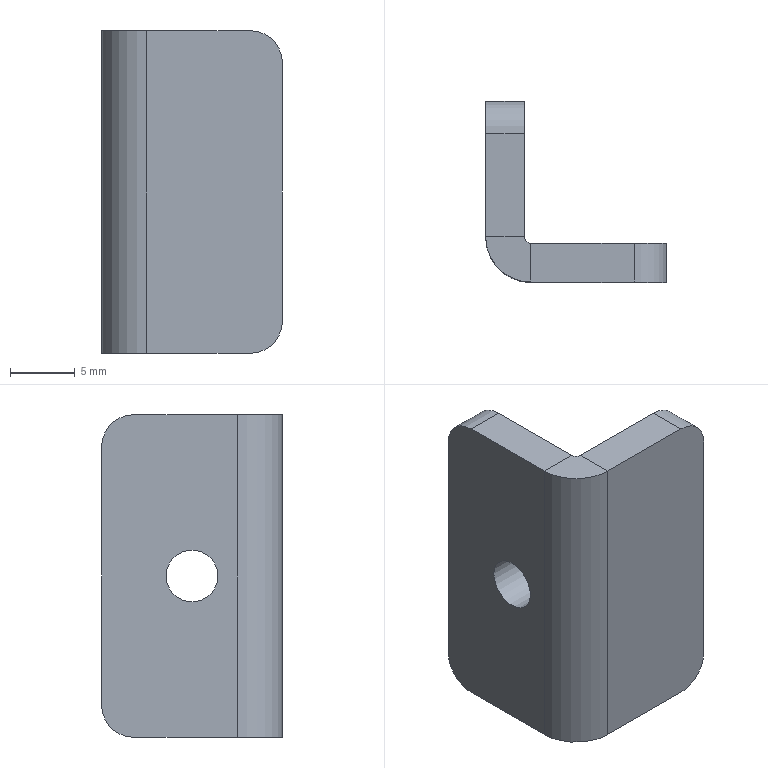Part | STEP file | Q7C0513 | 1 solid | 19 faces | box 14 x 14 x 25 mm | volume 1757 mm3 | plane 12 | cylinder 7 | commonest cylinder face diameters 5 x4 1 x1 4 x1 7 x1
STEP:
#1=CARTESIAN_POINT('',(0.,0.,0.));
#2=DIRECTION('',(0.,0.,1.));
#3=DIRECTION('',(1.,0.,0.));
#4=AXIS2_PLACEMENT_3D('',#1,#2,#3);
#5=CARTESIAN_POINT('',(0.,3.5,12.5));
#6=VERTEX_POINT('',#5);
#7=CARTESIAN_POINT('',(3.,3.5,12.5));
#8=VERTEX_POINT('',#7);
#9=CARTESIAN_POINT('',(0.,3.5,12.5));
#10=DIRECTION('',(1.,0.,0.));
#11=VECTOR('',#10,1.);
#12=LINE('',#9,#11);
#13=CARTESIAN_POINT('',(0.,3.5,12.5));
#14=DIRECTION('',(0.,0.,1.));
#15=DIRECTION('',(1.,0.,0.));
#16=AXIS2_PLACEMENT_3D('',#13,#14,#15);
#17=PLANE('',#16);
#18=CARTESIAN_POINT('',(0.,0.));
#19=DIRECTION('',(1.,0.));
#20=VECTOR('',#19,1.);
#21=LINE('',#18,#20);
#22=(GEOMETRIC_REPRESENTATION_CONTEXT(2)PARAMETRIC_REPRESENTATION_CONTEXT()REPRESENTATION_CONTEXT('',''));
#23=DEFINITIONAL_REPRESENTATION('',(#21),#22);
#24=PCURVE('',#17,#23);
#25=CARTESIAN_POINT('',(3.5,3.,12.5));
#26=DIRECTION('',(0.,0.,1.));
#27=DIRECTION('',(1.,0.,0.));
#28=AXIS2_PLACEMENT_3D('',#25,#26,#27);
#29=PLANE('',#28);
#30=CARTESIAN_POINT('',(-3.5,0.5));
#31=DIRECTION('',(1.,0.));
#32=VECTOR('',#31,1.);
#33=LINE('',#30,#32);
#34=(GEOMETRIC_REPRESENTATION_CONTEXT(2)PARAMETRIC_REPRESENTATION_CONTEXT()REPRESENTATION_CONTEXT('',''));
#35=DEFINITIONAL_REPRESENTATION('',(#33),#34);
#36=PCURVE('',#29,#35);
#37=SURFACE_CURVE('',#12,(#24,#36),.PCURVE_S1.);
#38=EDGE_CURVE('',#6,#8,#37,.T.);
#39=ORIENTED_EDGE('',*,*,#38,.F.);
#40=CARTESIAN_POINT('',(3.5,0.,12.5));
#41=VERTEX_POINT('',#40);
#42=CARTESIAN_POINT('',(3.5,3.5,12.5));
#43=DIRECTION('',(0.,0.,1.));
#44=DIRECTION('',(-1.,0.,0.));
#45=AXIS2_PLACEMENT_3D('',#42,#43,#44);
#46=CIRCLE('',#45,3.5);
#47=CARTESIAN_POINT('',(3.5,0.));
#48=DIRECTION('',(-1.,0.));
#49=AXIS2_PLACEMENT_2D('',#47,#48);
#50=CIRCLE('',#49,3.5);
#51=(GEOMETRIC_REPRESENTATION_CONTEXT(2)PARAMETRIC_REPRESENTATION_CONTEXT()REPRESENTATION_CONTEXT('',''));
#52=DEFINITIONAL_REPRESENTATION('',(#50),#51);
#53=PCURVE('',#17,#52);
#54=CARTESIAN_POINT('',(3.5,3.5,12.5));
#55=DIRECTION('',(0.,0.,-1.));
#56=DIRECTION('',(-1.,0.,0.));
#57=AXIS2_PLACEMENT_3D('',#54,#55,#56);
#58=CYLINDRICAL_SURFACE('',#57,3.5);
#59=CARTESIAN_POINT('',(6.283,0.));
#60=DIRECTION('',(-1.,0.));
#61=VECTOR('',#60,1.);
#62=LINE('',#59,#61);
#63=(GEOMETRIC_REPRESENTATION_CONTEXT(2)PARAMETRIC_REPRESENTATION_CONTEXT()REPRESENTATION_CONTEXT('',''));
#64=DEFINITIONAL_REPRESENTATION('',(#62),#63);
#65=PCURVE('',#58,#64);
#66=SURFACE_CURVE('',#46,(#53,#65),.PCURVE_S1.);
#67=EDGE_CURVE('',#6,#41,#66,.T.);
#68=ORIENTED_EDGE('',*,*,#67,.T.);
#69=CARTESIAN_POINT('',(3.5,3.,12.5));
#70=VERTEX_POINT('',#69);
#71=CARTESIAN_POINT('',(3.5,3.,12.5));
#72=DIRECTION('',(0.,-1.,0.));
#73=VECTOR('',#72,1.);
#74=LINE('',#71,#73);
#75=CARTESIAN_POINT('',(3.5,-0.5));
#76=DIRECTION('',(0.,-1.));
#77=VECTOR('',#76,1.);
#78=LINE('',#75,#77);
#79=(GEOMETRIC_REPRESENTATION_CONTEXT(2)PARAMETRIC_REPRESENTATION_CONTEXT()REPRESENTATION_CONTEXT('',''));
#80=DEFINITIONAL_REPRESENTATION('',(#78),#79);
#81=PCURVE('',#17,#80);
#82=CARTESIAN_POINT('',(3.5,3.5,12.5));
#83=DIRECTION('',(0.,0.,1.));
#84=DIRECTION('',(1.,0.,0.));
#85=AXIS2_PLACEMENT_3D('',#82,#83,#84);
#86=PLANE('',#85);
#87=CARTESIAN_POINT('',(0.,-0.5));
#88=DIRECTION('',(0.,-1.));
#89=VECTOR('',#88,1.);
#90=LINE('',#87,#89);
#91=(GEOMETRIC_REPRESENTATION_CONTEXT(2)PARAMETRIC_REPRESENTATION_CONTEXT()REPRESENTATION_CONTEXT('',''));
#92=DEFINITIONAL_REPRESENTATION('',(#90),#91);
#93=PCURVE('',#86,#92);
#94=SURFACE_CURVE('',#74,(#81,#93),.PCURVE_S1.);
#95=EDGE_CURVE('',#70,#41,#94,.T.);
#96=ORIENTED_EDGE('',*,*,#95,.F.);
#97=CARTESIAN_POINT('',(3.5,3.5,12.5));
#98=DIRECTION('',(0.,0.,1.));
#99=DIRECTION('',(1.,0.,0.));
#100=AXIS2_PLACEMENT_3D('',#97,#98,#99);
#101=CIRCLE('',#100,0.5);
#102=CARTESIAN_POINT('',(3.5,0.));
#103=DIRECTION('',(1.,0.));
#104=AXIS2_PLACEMENT_2D('',#102,#103);
#105=CIRCLE('',#104,0.5);
#106=(GEOMETRIC_REPRESENTATION_CONTEXT(2)PARAMETRIC_REPRESENTATION_CONTEXT()REPRESENTATION_CONTEXT('',''));
#107=DEFINITIONAL_REPRESENTATION('',(#105),#106);
#108=PCURVE('',#17,#107);
#109=CARTESIAN_POINT('',(3.5,3.5,12.5));
#110=DIRECTION('',(0.,0.,-1.));
#111=DIRECTION('',(-1.,0.,0.));
#112=AXIS2_PLACEMENT_3D('',#109,#110,#111);
#113=CYLINDRICAL_SURFACE('',#112,0.5);
#114=CARTESIAN_POINT('',(9.425,0.));
#115=DIRECTION('',(-1.,0.));
#116=VECTOR('',#115,1.);
#117=LINE('',#114,#116);
#118=(GEOMETRIC_REPRESENTATION_CONTEXT(2)PARAMETRIC_REPRESENTATION_CONTEXT()REPRESENTATION_CONTEXT('',''));
#119=DEFINITIONAL_REPRESENTATION('',(#117),#118);
#120=PCURVE('',#113,#119);
#121=SURFACE_CURVE('',#101,(#108,#120),.PCURVE_S1.);
#122=EDGE_CURVE('',#8,#70,#121,.T.);
#123=ORIENTED_EDGE('',*,*,#122,.F.);
#124=EDGE_LOOP('',(#39,#68,#96,#123));
#125=FACE_BOUND('',#124,.T.);
#126=ADVANCED_FACE('',(#125),#17,.T.);
#127=CARTESIAN_POINT('',(3.,11.5,12.5));
#128=VERTEX_POINT('',#127);
#129=CARTESIAN_POINT('',(3.,14.,12.5));
#130=DIRECTION('',(0.,-1.,0.));
#131=VECTOR('',#130,1.);
#132=LINE('',#129,#131);
#133=CARTESIAN_POINT('',(-0.5,11.));
#134=DIRECTION('',(0.,-1.));
#135=VECTOR('',#134,1.);
#136=LINE('',#133,#135);
#137=(GEOMETRIC_REPRESENTATION_CONTEXT(2)PARAMETRIC_REPRESENTATION_CONTEXT()REPRESENTATION_CONTEXT('',''));
#138=DEFINITIONAL_REPRESENTATION('',(#136),#137);
#139=PCURVE('',#29,#138);
#140=CARTESIAN_POINT('',(3.,14.,12.5));
#141=DIRECTION('',(1.,0.,0.));
#142=DIRECTION('',(0.,1.,0.));
#143=AXIS2_PLACEMENT_3D('',#140,#141,#142);
#144=PLANE('',#143);
#145=CARTESIAN_POINT('',(0.,0.));
#146=DIRECTION('',(-1.,0.));
#147=VECTOR('',#146,1.);
#148=LINE('',#145,#147);
#149=(GEOMETRIC_REPRESENTATION_CONTEXT(2)PARAMETRIC_REPRESENTATION_CONTEXT()REPRESENTATION_CONTEXT('',''));
#150=DEFINITIONAL_REPRESENTATION('',(#148),#149);
#151=PCURVE('',#144,#150);
#152=SURFACE_CURVE('',#132,(#139,#151),.PCURVE_S1.);
#153=EDGE_CURVE('',#128,#8,#152,.T.);
#154=ORIENTED_EDGE('',*,*,#153,.F.);
#155=CARTESIAN_POINT('',(0.,11.5,12.5));
#156=VERTEX_POINT('',#155);
#157=CARTESIAN_POINT('',(3.5,11.5,12.5));
#158=DIRECTION('',(-1.,0.,0.));
#159=VECTOR('',#158,1.);
#160=LINE('',#157,#159);
#161=CARTESIAN_POINT('',(0.,8.5));
#162=DIRECTION('',(-1.,0.));
#163=VECTOR('',#162,1.);
#164=LINE('',#161,#163);
#165=(GEOMETRIC_REPRESENTATION_CONTEXT(2)PARAMETRIC_REPRESENTATION_CONTEXT()REPRESENTATION_CONTEXT('',''));
#166=DEFINITIONAL_REPRESENTATION('',(#164),#165);
#167=PCURVE('',#29,#166);
#168=CARTESIAN_POINT('',(0.,11.5,10.));
#169=DIRECTION('',(1.,0.,0.));
#170=DIRECTION('',(0.,1.,0.));
#171=AXIS2_PLACEMENT_3D('',#168,#169,#170);
#172=CYLINDRICAL_SURFACE('',#171,2.5);
#173=CARTESIAN_POINT('',(1.571,3.5));
#174=DIRECTION('',(0.,-1.));
#175=VECTOR('',#174,1.);
#176=LINE('',#173,#175);
#177=(GEOMETRIC_REPRESENTATION_CONTEXT(2)PARAMETRIC_REPRESENTATION_CONTEXT()REPRESENTATION_CONTEXT('',''));
#178=DEFINITIONAL_REPRESENTATION('',(#176),#177);
#179=PCURVE('',#172,#178);
#180=SURFACE_CURVE('',#160,(#167,#179),.PCURVE_S1.);
#181=EDGE_CURVE('',#128,#156,#180,.T.);
#182=ORIENTED_EDGE('',*,*,#181,.T.);
#183=CARTESIAN_POINT('',(0.,14.,12.5));
#184=DIRECTION('',(0.,-1.,0.));
#185=VECTOR('',#184,1.);
#186=LINE('',#183,#185);
#187=CARTESIAN_POINT('',(-3.5,11.));
#188=DIRECTION('',(0.,-1.));
#189=VECTOR('',#188,1.);
#190=LINE('',#187,#189);
#191=(GEOMETRIC_REPRESENTATION_CONTEXT(2)PARAMETRIC_REPRESENTATION_CONTEXT()REPRESENTATION_CONTEXT('',''));
#192=DEFINITIONAL_REPRESENTATION('',(#190),#191);
#193=PCURVE('',#29,#192);
#194=CARTESIAN_POINT('',(0.,14.,12.5));
#195=DIRECTION('',(1.,0.,0.));
#196=DIRECTION('',(0.,1.,0.));
#197=AXIS2_PLACEMENT_3D('',#194,#195,#196);
#198=PLANE('',#197);
#199=CARTESIAN_POINT('',(0.,0.));
#200=DIRECTION('',(-1.,0.));
#201=VECTOR('',#200,1.);
#202=LINE('',#199,#201);
#203=(GEOMETRIC_REPRESENTATION_CONTEXT(2)PARAMETRIC_REPRESENTATION_CONTEXT()REPRESENTATION_CONTEXT('',''));
#204=DEFINITIONAL_REPRESENTATION('',(#202),#203);
#205=PCURVE('',#198,#204);
#206=SURFACE_CURVE('',#186,(#193,#205),.PCURVE_S1.);
#207=EDGE_CURVE('',#156,#6,#206,.T.);
#208=ORIENTED_EDGE('',*,*,#207,.T.);
#209=ORIENTED_EDGE('',*,*,#38,.T.);
#210=EDGE_LOOP('',(#154,#182,#208,#209));
#211=FACE_BOUND('',#210,.T.);
#212=ADVANCED_FACE('',(#211),#29,.T.);
#213=CARTESIAN_POINT('',(3.5,0.,-12.5));
#214=VERTEX_POINT('',#213);
#215=CARTESIAN_POINT('',(3.5,3.,-12.5));
#216=VERTEX_POINT('',#215);
#217=CARTESIAN_POINT('',(3.5,0.,-12.5));
#218=DIRECTION('',(0.,1.,0.));
#219=VECTOR('',#218,1.);
#220=LINE('',#217,#219);
#221=CARTESIAN_POINT('',(3.5,0.,-12.5));
#222=DIRECTION('',(0.,0.,-1.));
#223=DIRECTION('',(-1.,0.,0.));
#224=AXIS2_PLACEMENT_3D('',#221,#222,#223);
#225=PLANE('',#224);
#226=CARTESIAN_POINT('',(0.,0.));
#227=DIRECTION('',(0.,1.));
#228=VECTOR('',#227,1.);
#229=LINE('',#226,#228);
#230=(GEOMETRIC_REPRESENTATION_CONTEXT(2)PARAMETRIC_REPRESENTATION_CONTEXT()REPRESENTATION_CONTEXT('',''));
#231=DEFINITIONAL_REPRESENTATION('',(#229),#230);
#232=PCURVE('',#225,#231);
#233=CARTESIAN_POINT('',(3.,3.5,-12.5));
#234=DIRECTION('',(0.,0.,-1.));
#235=DIRECTION('',(-1.,0.,0.));
#236=AXIS2_PLACEMENT_3D('',#233,#234,#235);
#237=PLANE('',#236);
#238=CARTESIAN_POINT('',(-0.5,-3.5));
#239=DIRECTION('',(0.,1.));
#240=VECTOR('',#239,1.);
#241=LINE('',#238,#240);
#242=(GEOMETRIC_REPRESENTATION_CONTEXT(2)PARAMETRIC_REPRESENTATION_CONTEXT()REPRESENTATION_CONTEXT('',''));
#243=DEFINITIONAL_REPRESENTATION('',(#241),#242);
#244=PCURVE('',#237,#243);
#245=SURFACE_CURVE('',#220,(#232,#244),.PCURVE_S1.);
#246=EDGE_CURVE('',#214,#216,#245,.T.);
#247=ORIENTED_EDGE('',*,*,#246,.F.);
#248=CARTESIAN_POINT('',(0.,3.5,-12.5));
#249=VERTEX_POINT('',#248);
#250=CARTESIAN_POINT('',(3.5,3.5,-12.5));
#251=DIRECTION('',(0.,0.,1.));
#252=DIRECTION('',(-1.,0.,0.));
#253=AXIS2_PLACEMENT_3D('',#250,#251,#252);
#254=CIRCLE('',#253,3.5);
#255=CARTESIAN_POINT('',(3.5,3.5));
#256=CARTESIAN_POINT('',(3.5,-2.562));
#257=CARTESIAN_POINT('',(-1.75,0.4689));
#258=CARTESIAN_POINT('',(-7.,3.5));
#259=CARTESIAN_POINT('',(-1.75,6.531));
#260=CARTESIAN_POINT('',(3.5,9.562));
#261=CARTESIAN_POINT('',(3.5,3.5));
#262=(BOUNDED_CURVE()B_SPLINE_CURVE(2,(#255,#256,#257,#258,#259,#260,#261),.UNSPECIFIED.,.T.,.F.)B_SPLINE_CURVE_WITH_KNOTS((1,2,2,2,2,1),(-2.094,0.,2.094,4.189,6.283,8.378),.UNSPECIFIED.)CURVE()GEOMETRIC_REPRESENTATION_ITEM()RATIONAL_B_SPLINE_CURVE((1.,0.5,1.,0.5,1.,0.5,1.))REPRESENTATION_ITEM(''));
#263=(GEOMETRIC_REPRESENTATION_CONTEXT(2)PARAMETRIC_REPRESENTATION_CONTEXT()REPRESENTATION_CONTEXT('',''));
#264=DEFINITIONAL_REPRESENTATION('',(#262),#263);
#265=PCURVE('',#225,#264);
#266=CARTESIAN_POINT('',(6.283,25.));
#267=DIRECTION('',(-1.,0.));
#268=VECTOR('',#267,1.);
#269=LINE('',#266,#268);
#270=(GEOMETRIC_REPRESENTATION_CONTEXT(2)PARAMETRIC_REPRESENTATION_CONTEXT()REPRESENTATION_CONTEXT('',''));
#271=DEFINITIONAL_REPRESENTATION('',(#269),#270);
#272=PCURVE('',#58,#271);
#273=SURFACE_CURVE('',#254,(#265,#272),.PCURVE_S1.);
#274=EDGE_CURVE('',#249,#214,#273,.T.);
#275=ORIENTED_EDGE('',*,*,#274,.F.);
#276=CARTESIAN_POINT('',(3.,3.5,-12.5));
#277=VERTEX_POINT('',#276);
#278=CARTESIAN_POINT('',(3.,3.5,-12.5));
#279=DIRECTION('',(-1.,0.,0.));
#280=VECTOR('',#279,1.);
#281=LINE('',#278,#280);
#282=CARTESIAN_POINT('',(0.5,3.5));
#283=DIRECTION('',(1.,0.));
#284=VECTOR('',#283,1.);
#285=LINE('',#282,#284);
#286=(GEOMETRIC_REPRESENTATION_CONTEXT(2)PARAMETRIC_REPRESENTATION_CONTEXT()REPRESENTATION_CONTEXT('',''));
#287=DEFINITIONAL_REPRESENTATION('',(#285),#286);
#288=PCURVE('',#225,#287);
#289=CARTESIAN_POINT('',(3.5,3.5,-12.5));
#290=DIRECTION('',(0.,0.,1.));
#291=DIRECTION('',(1.,0.,0.));
#292=AXIS2_PLACEMENT_3D('',#289,#290,#291);
#293=PLANE('',#292);
#294=CARTESIAN_POINT('',(-0.5,0.));
#295=DIRECTION('',(-1.,0.));
#296=VECTOR('',#295,1.);
#297=LINE('',#294,#296);
#298=(GEOMETRIC_REPRESENTATION_CONTEXT(2)PARAMETRIC_REPRESENTATION_CONTEXT()REPRESENTATION_CONTEXT('',''));
#299=DEFINITIONAL_REPRESENTATION('',(#297),#298);
#300=PCURVE('',#293,#299);
#301=SURFACE_CURVE('',#281,(#288,#300),.PCURVE_S1.);
#302=EDGE_CURVE('',#277,#249,#301,.T.);
#303=ORIENTED_EDGE('',*,*,#302,.F.);
#304=CARTESIAN_POINT('',(3.5,3.5,-12.5));
#305=DIRECTION('',(0.,0.,1.));
#306=DIRECTION('',(1.,0.,0.));
#307=AXIS2_PLACEMENT_3D('',#304,#305,#306);
#308=CIRCLE('',#307,0.5);
#309=CARTESIAN_POINT('',(-0.5,3.5));
#310=CARTESIAN_POINT('',(-0.5,4.366));
#311=CARTESIAN_POINT('',(0.25,3.933));
#312=CARTESIAN_POINT('',(1.,3.5));
#313=CARTESIAN_POINT('',(0.25,3.067));
#314=CARTESIAN_POINT('',(-0.5,2.634));
#315=CARTESIAN_POINT('',(-0.5,3.5));
#316=(BOUNDED_CURVE()B_SPLINE_CURVE(2,(#309,#310,#311,#312,#313,#314,#315),.UNSPECIFIED.,.T.,.F.)B_SPLINE_CURVE_WITH_KNOTS((1,2,2,2,2,1),(-2.094,0.,2.094,4.189,6.283,8.378),.UNSPECIFIED.)CURVE()GEOMETRIC_REPRESENTATION_ITEM()RATIONAL_B_SPLINE_CURVE((1.,0.5,1.,0.5,1.,0.5,1.))REPRESENTATION_ITEM(''));
#317=(GEOMETRIC_REPRESENTATION_CONTEXT(2)PARAMETRIC_REPRESENTATION_CONTEXT()REPRESENTATION_CONTEXT('',''));
#318=DEFINITIONAL_REPRESENTATION('',(#316),#317);
#319=PCURVE('',#225,#318);
#320=CARTESIAN_POINT('',(9.425,25.));
#321=DIRECTION('',(-1.,0.));
#322=VECTOR('',#321,1.);
#323=LINE('',#320,#322);
#324=(GEOMETRIC_REPRESENTATION_CONTEXT(2)PARAMETRIC_REPRESENTATION_CONTEXT()REPRESENTATION_CONTEXT('',''));
#325=DEFINITIONAL_REPRESENTATION('',(#323),#324);
#326=PCURVE('',#113,#325);
#327=SURFACE_CURVE('',#308,(#319,#326),.PCURVE_S1.);
#328=EDGE_CURVE('',#277,#216,#327,.T.);
#329=ORIENTED_EDGE('',*,*,#328,.T.);
#330=EDGE_LOOP('',(#247,#275,#303,#329));
#331=FACE_BOUND('',#330,.T.);
#332=ADVANCED_FACE('',(#331),#225,.T.);
#333=CARTESIAN_POINT('',(11.5,3.,-12.5));
#334=VERTEX_POINT('',#333);
#335=CARTESIAN_POINT('',(3.5,3.,-12.5));
#336=DIRECTION('',(1.,0.,0.));
#337=VECTOR('',#336,1.);
#338=LINE('',#335,#337);
#339=CARTESIAN_POINT('',(-0.5,-0.5));
#340=DIRECTION('',(-1.,0.));
#341=VECTOR('',#340,1.);
#342=LINE('',#339,#341);
#343=(GEOMETRIC_REPRESENTATION_CONTEXT(2)PARAMETRIC_REPRESENTATION_CONTEXT()REPRESENTATION_CONTEXT('',''));
#344=DEFINITIONAL_REPRESENTATION('',(#342),#343);
#345=PCURVE('',#237,#344);
#346=CARTESIAN_POINT('',(3.5,3.,12.5));
#347=DIRECTION('',(0.,1.,0.));
#348=DIRECTION('',(0.,0.,1.));
#349=AXIS2_PLACEMENT_3D('',#346,#347,#348);
#350=PLANE('',#349);
#351=CARTESIAN_POINT('',(-25.,0.));
#352=DIRECTION('',(0.,1.));
#353=VECTOR('',#352,1.);
#354=LINE('',#351,#353);
#355=(GEOMETRIC_REPRESENTATION_CONTEXT(2)PARAMETRIC_REPRESENTATION_CONTEXT()REPRESENTATION_CONTEXT('',''));
#356=DEFINITIONAL_REPRESENTATION('',(#354),#355);
#357=PCURVE('',#350,#356);
#358=SURFACE_CURVE('',#338,(#345,#357),.PCURVE_S1.);
#359=EDGE_CURVE('',#216,#334,#358,.T.);
#360=ORIENTED_EDGE('',*,*,#359,.T.);
#361=CARTESIAN_POINT('',(11.5,0.,-12.5));
#362=VERTEX_POINT('',#361);
#363=CARTESIAN_POINT('',(11.5,3.5,-12.5));
#364=DIRECTION('',(0.,-1.,0.));
#365=VECTOR('',#364,1.);
#366=LINE('',#363,#365);
#367=CARTESIAN_POINT('',(-8.5,0.));
#368=DIRECTION('',(0.,-1.));
#369=VECTOR('',#368,1.);
#370=LINE('',#367,#369);
#371=(GEOMETRIC_REPRESENTATION_CONTEXT(2)PARAMETRIC_REPRESENTATION_CONTEXT()REPRESENTATION_CONTEXT('',''));
#372=DEFINITIONAL_REPRESENTATION('',(#370),#371);
#373=PCURVE('',#237,#372);
#374=CARTESIAN_POINT('',(11.5,3.5,-10.));
#375=DIRECTION('',(0.,-1.,0.));
#376=DIRECTION('',(0.,0.,-1.));
#377=AXIS2_PLACEMENT_3D('',#374,#375,#376);
#378=CYLINDRICAL_SURFACE('',#377,2.5);
#379=CARTESIAN_POINT('',(0.,0.));
#380=DIRECTION('',(0.,1.));
#381=VECTOR('',#380,1.);
#382=LINE('',#379,#381);
#383=(GEOMETRIC_REPRESENTATION_CONTEXT(2)PARAMETRIC_REPRESENTATION_CONTEXT()REPRESENTATION_CONTEXT('',''));
#384=DEFINITIONAL_REPRESENTATION('',(#382),#383);
#385=PCURVE('',#378,#384);
#386=SURFACE_CURVE('',#366,(#373,#385),.PCURVE_S1.);
#387=EDGE_CURVE('',#334,#362,#386,.T.);
#388=ORIENTED_EDGE('',*,*,#387,.T.);
#389=CARTESIAN_POINT('',(3.5,0.,-12.5));
#390=DIRECTION('',(1.,0.,0.));
#391=VECTOR('',#390,1.);
#392=LINE('',#389,#391);
#393=CARTESIAN_POINT('',(-0.5,-3.5));
#394=DIRECTION('',(-1.,0.));
#395=VECTOR('',#394,1.);
#396=LINE('',#393,#395);
#397=(GEOMETRIC_REPRESENTATION_CONTEXT(2)PARAMETRIC_REPRESENTATION_CONTEXT()REPRESENTATION_CONTEXT('',''));
#398=DEFINITIONAL_REPRESENTATION('',(#396),#397);
#399=PCURVE('',#237,#398);
#400=CARTESIAN_POINT('',(3.5,0.,12.5));
#401=DIRECTION('',(0.,1.,0.));
#402=DIRECTION('',(0.,0.,1.));
#403=AXIS2_PLACEMENT_3D('',#400,#401,#402);
#404=PLANE('',#403);
#405=CARTESIAN_POINT('',(-25.,0.));
#406=DIRECTION('',(0.,1.));
#407=VECTOR('',#406,1.);
#408=LINE('',#405,#407);
#409=(GEOMETRIC_REPRESENTATION_CONTEXT(2)PARAMETRIC_REPRESENTATION_CONTEXT()REPRESENTATION_CONTEXT('',''));
#410=DEFINITIONAL_REPRESENTATION('',(#408),#409);
#411=PCURVE('',#404,#410);
#412=SURFACE_CURVE('',#392,(#399,#411),.PCURVE_S1.);
#413=EDGE_CURVE('',#214,#362,#412,.T.);
#414=ORIENTED_EDGE('',*,*,#413,.F.);
#415=ORIENTED_EDGE('',*,*,#246,.T.);
#416=EDGE_LOOP('',(#360,#388,#414,#415));
#417=FACE_BOUND('',#416,.T.);
#418=ADVANCED_FACE('',(#417),#237,.T.);
#419=ORIENTED_EDGE('',*,*,#413,.T.);
#420=CARTESIAN_POINT('',(14.,0.,-10.));
#421=VERTEX_POINT('',#420);
#422=CARTESIAN_POINT('',(11.5,0.,-10.));
#423=DIRECTION('',(0.,-1.,0.));
#424=DIRECTION('',(0.,0.,1.));
#425=AXIS2_PLACEMENT_3D('',#422,#423,#424);
#426=CIRCLE('',#425,2.5);
#427=CARTESIAN_POINT('',(-20.,8.));
#428=CARTESIAN_POINT('',(-20.,3.67));
#429=CARTESIAN_POINT('',(-23.75,5.835));
#430=CARTESIAN_POINT('',(-27.5,8.));
#431=CARTESIAN_POINT('',(-23.75,10.165));
#432=CARTESIAN_POINT('',(-20.,12.33));
#433=CARTESIAN_POINT('',(-20.,8.));
#434=(BOUNDED_CURVE()B_SPLINE_CURVE(2,(#427,#428,#429,#430,#431,#432,#433),.UNSPECIFIED.,.T.,.F.)B_SPLINE_CURVE_WITH_KNOTS((1,2,2,2,2,1),(-2.094,0.,2.094,4.189,6.283,8.378),.UNSPECIFIED.)CURVE()GEOMETRIC_REPRESENTATION_ITEM()RATIONAL_B_SPLINE_CURVE((1.,0.5,1.,0.5,1.,0.5,1.))REPRESENTATION_ITEM(''));
#435=(GEOMETRIC_REPRESENTATION_CONTEXT(2)PARAMETRIC_REPRESENTATION_CONTEXT()REPRESENTATION_CONTEXT('',''));
#436=DEFINITIONAL_REPRESENTATION('',(#434),#435);
#437=PCURVE('',#404,#436);
#438=CARTESIAN_POINT('',(-3.142,3.5));
#439=DIRECTION('',(1.,0.));
#440=VECTOR('',#439,1.);
#441=LINE('',#438,#440);
#442=(GEOMETRIC_REPRESENTATION_CONTEXT(2)PARAMETRIC_REPRESENTATION_CONTEXT()REPRESENTATION_CONTEXT('',''));
#443=DEFINITIONAL_REPRESENTATION('',(#441),#442);
#444=PCURVE('',#378,#443);
#445=SURFACE_CURVE('',#426,(#437,#444),.PCURVE_S1.);
#446=EDGE_CURVE('',#362,#421,#445,.T.);
#447=ORIENTED_EDGE('',*,*,#446,.T.);
#448=CARTESIAN_POINT('',(14.,0.,10.));
#449=VERTEX_POINT('',#448);
#450=CARTESIAN_POINT('',(14.,0.,12.5));
#451=DIRECTION('',(0.,0.,-1.));
#452=VECTOR('',#451,1.);
#453=LINE('',#450,#452);
#454=CARTESIAN_POINT('',(0.,10.5));
#455=DIRECTION('',(-1.,0.));
#456=VECTOR('',#455,1.);
#457=LINE('',#454,#456);
#458=(GEOMETRIC_REPRESENTATION_CONTEXT(2)PARAMETRIC_REPRESENTATION_CONTEXT()REPRESENTATION_CONTEXT('',''));
#459=DEFINITIONAL_REPRESENTATION('',(#457),#458);
#460=PCURVE('',#404,#459);
#461=CARTESIAN_POINT('',(14.,3.,12.5));
#462=DIRECTION('',(1.,0.,0.));
#463=DIRECTION('',(0.,0.,-1.));
#464=AXIS2_PLACEMENT_3D('',#461,#462,#463);
#465=PLANE('',#464);
#466=CARTESIAN_POINT('',(0.,-3.));
#467=DIRECTION('',(1.,0.));
#468=VECTOR('',#467,1.);
#469=LINE('',#466,#468);
#470=(GEOMETRIC_REPRESENTATION_CONTEXT(2)PARAMETRIC_REPRESENTATION_CONTEXT()REPRESENTATION_CONTEXT('',''));
#471=DEFINITIONAL_REPRESENTATION('',(#469),#470);
#472=PCURVE('',#465,#471);
#473=SURFACE_CURVE('',#453,(#460,#472),.PCURVE_S1.);
#474=EDGE_CURVE('',#449,#421,#473,.T.);
#475=ORIENTED_EDGE('',*,*,#474,.F.);
#476=CARTESIAN_POINT('',(11.5,0.,12.5));
#477=VERTEX_POINT('',#476);
#478=CARTESIAN_POINT('',(11.5,0.,10.));
#479=DIRECTION('',(0.,-1.,0.));
#480=DIRECTION('',(0.,0.,1.));
#481=AXIS2_PLACEMENT_3D('',#478,#479,#480);
#482=CIRCLE('',#481,2.5);
#483=CARTESIAN_POINT('',(0.,8.));
#484=CARTESIAN_POINT('',(0.,3.67));
#485=CARTESIAN_POINT('',(-3.75,5.835));
#486=CARTESIAN_POINT('',(-7.5,8.));
#487=CARTESIAN_POINT('',(-3.75,10.165));
#488=CARTESIAN_POINT('',(0.,12.33));
#489=CARTESIAN_POINT('',(0.,8.));
#490=(BOUNDED_CURVE()B_SPLINE_CURVE(2,(#483,#484,#485,#486,#487,#488,#489),.UNSPECIFIED.,.T.,.F.)B_SPLINE_CURVE_WITH_KNOTS((1,2,2,2,2,1),(-2.094,0.,2.094,4.189,6.283,8.378),.UNSPECIFIED.)CURVE()GEOMETRIC_REPRESENTATION_ITEM()RATIONAL_B_SPLINE_CURVE((1.,0.5,1.,0.5,1.,0.5,1.))REPRESENTATION_ITEM(''));
#491=(GEOMETRIC_REPRESENTATION_CONTEXT(2)PARAMETRIC_REPRESENTATION_CONTEXT()REPRESENTATION_CONTEXT('',''));
#492=DEFINITIONAL_REPRESENTATION('',(#490),#491);
#493=PCURVE('',#404,#492);
#494=CARTESIAN_POINT('',(11.5,3.,10.));
#495=DIRECTION('',(0.,-1.,0.));
#496=DIRECTION('',(0.,0.,-1.));
#497=AXIS2_PLACEMENT_3D('',#494,#495,#496);
#498=CYLINDRICAL_SURFACE('',#497,2.5);
#499=CARTESIAN_POINT('',(-3.142,3.));
#500=DIRECTION('',(1.,0.));
#501=VECTOR('',#500,1.);
#502=LINE('',#499,#501);
#503=(GEOMETRIC_REPRESENTATION_CONTEXT(2)PARAMETRIC_REPRESENTATION_CONTEXT()REPRESENTATION_CONTEXT('',''));
#504=DEFINITIONAL_REPRESENTATION('',(#502),#503);
#505=PCURVE('',#498,#504);
#506=SURFACE_CURVE('',#482,(#493,#505),.PCURVE_S1.);
#507=EDGE_CURVE('',#449,#477,#506,.T.);
#508=ORIENTED_EDGE('',*,*,#507,.T.);
#509=CARTESIAN_POINT('',(3.5,0.,12.5));
#510=DIRECTION('',(1.,0.,0.));
#511=VECTOR('',#510,1.);
#512=LINE('',#509,#511);
#513=CARTESIAN_POINT('',(0.,0.));
#514=DIRECTION('',(0.,1.));
#515=VECTOR('',#514,1.);
#516=LINE('',#513,#515);
#517=(GEOMETRIC_REPRESENTATION_CONTEXT(2)PARAMETRIC_REPRESENTATION_CONTEXT()REPRESENTATION_CONTEXT('',''));
#518=DEFINITIONAL_REPRESENTATION('',(#516),#517);
#519=PCURVE('',#404,#518);
#520=CARTESIAN_POINT('',(0.,-3.5));
#521=DIRECTION('',(1.,0.));
#522=VECTOR('',#521,1.);
#523=LINE('',#520,#522);
#524=(GEOMETRIC_REPRESENTATION_CONTEXT(2)PARAMETRIC_REPRESENTATION_CONTEXT()REPRESENTATION_CONTEXT('',''));
#525=DEFINITIONAL_REPRESENTATION('',(#523),#524);
#526=PCURVE('',#86,#525);
#527=SURFACE_CURVE('',#512,(#519,#526),.PCURVE_S1.);
#528=EDGE_CURVE('',#41,#477,#527,.T.);
#529=ORIENTED_EDGE('',*,*,#528,.F.);
#530=CARTESIAN_POINT('',(3.5,0.,12.5));
#531=DIRECTION('',(0.,0.,-1.));
#532=VECTOR('',#531,1.);
#533=LINE('',#530,#532);
#534=CARTESIAN_POINT('',(0.,0.));
#535=DIRECTION('',(-1.,0.));
#536=VECTOR('',#535,1.);
#537=LINE('',#534,#536);
#538=(GEOMETRIC_REPRESENTATION_CONTEXT(2)PARAMETRIC_REPRESENTATION_CONTEXT()REPRESENTATION_CONTEXT('',''));
#539=DEFINITIONAL_REPRESENTATION('',(#537),#538);
#540=PCURVE('',#404,#539);
#541=CARTESIAN_POINT('',(4.712,0.));
#542=DIRECTION('',(0.,1.));
#543=VECTOR('',#542,1.);
#544=LINE('',#541,#543);
#545=(GEOMETRIC_REPRESENTATION_CONTEXT(2)PARAMETRIC_REPRESENTATION_CONTEXT()REPRESENTATION_CONTEXT('',''));
#546=DEFINITIONAL_REPRESENTATION('',(#544),#545);
#547=PCURVE('',#58,#546);
#548=SURFACE_CURVE('',#533,(#540,#547),.PCURVE_S1.);
#549=EDGE_CURVE('',#41,#214,#548,.T.);
#550=ORIENTED_EDGE('',*,*,#549,.T.);
#551=EDGE_LOOP('',(#419,#447,#475,#508,#529,#550));
#552=FACE_BOUND('',#551,.T.);
#553=ADVANCED_FACE('',(#552),#404,.F.);
#554=ORIENTED_EDGE('',*,*,#474,.T.);
#555=CARTESIAN_POINT('',(14.,3.,-10.));
#556=VERTEX_POINT('',#555);
#557=CARTESIAN_POINT('',(14.,3.,-10.));
#558=DIRECTION('',(0.,1.,0.));
#559=VECTOR('',#558,1.);
#560=LINE('',#557,#559);
#561=CARTESIAN_POINT('',(22.5,0.));
#562=DIRECTION('',(0.,1.));
#563=VECTOR('',#562,1.);
#564=LINE('',#561,#563);
#565=(GEOMETRIC_REPRESENTATION_CONTEXT(2)PARAMETRIC_REPRESENTATION_CONTEXT()REPRESENTATION_CONTEXT('',''));
#566=DEFINITIONAL_REPRESENTATION('',(#564),#565);
#567=PCURVE('',#465,#566);
#568=CARTESIAN_POINT('',(1.571,0.5));
#569=DIRECTION('',(0.,-1.));
#570=VECTOR('',#569,1.);
#571=LINE('',#568,#570);
#572=(GEOMETRIC_REPRESENTATION_CONTEXT(2)PARAMETRIC_REPRESENTATION_CONTEXT()REPRESENTATION_CONTEXT('',''));
#573=DEFINITIONAL_REPRESENTATION('',(#571),#572);
#574=PCURVE('',#378,#573);
#575=SURFACE_CURVE('',#560,(#567,#574),.PCURVE_S1.);
#576=EDGE_CURVE('',#421,#556,#575,.T.);
#577=ORIENTED_EDGE('',*,*,#576,.T.);
#578=CARTESIAN_POINT('',(14.,3.,10.));
#579=VERTEX_POINT('',#578);
#580=CARTESIAN_POINT('',(14.,3.,12.5));
#581=DIRECTION('',(0.,0.,-1.));
#582=VECTOR('',#581,1.);
#583=LINE('',#580,#582);
#584=CARTESIAN_POINT('',(0.,0.));
#585=DIRECTION('',(1.,0.));
#586=VECTOR('',#585,1.);
#587=LINE('',#584,#586);
#588=(GEOMETRIC_REPRESENTATION_CONTEXT(2)PARAMETRIC_REPRESENTATION_CONTEXT()REPRESENTATION_CONTEXT('',''));
#589=DEFINITIONAL_REPRESENTATION('',(#587),#588);
#590=PCURVE('',#465,#589);
#591=CARTESIAN_POINT('',(0.,10.5));
#592=DIRECTION('',(-1.,0.));
#593=VECTOR('',#592,1.);
#594=LINE('',#591,#593);
#595=(GEOMETRIC_REPRESENTATION_CONTEXT(2)PARAMETRIC_REPRESENTATION_CONTEXT()REPRESENTATION_CONTEXT('',''));
#596=DEFINITIONAL_REPRESENTATION('',(#594),#595);
#597=PCURVE('',#350,#596);
#598=SURFACE_CURVE('',#583,(#590,#597),.PCURVE_S1.);
#599=EDGE_CURVE('',#579,#556,#598,.T.);
#600=ORIENTED_EDGE('',*,*,#599,.F.);
#601=CARTESIAN_POINT('',(14.,3.,10.));
#602=DIRECTION('',(0.,-1.,0.));
#603=VECTOR('',#602,1.);
#604=LINE('',#601,#603);
#605=CARTESIAN_POINT('',(2.5,0.));
#606=DIRECTION('',(0.,-1.));
#607=VECTOR('',#606,1.);
#608=LINE('',#605,#607);
#609=(GEOMETRIC_REPRESENTATION_CONTEXT(2)PARAMETRIC_REPRESENTATION_CONTEXT()REPRESENTATION_CONTEXT('',''));
#610=DEFINITIONAL_REPRESENTATION('',(#608),#609);
#611=PCURVE('',#465,#610);
#612=CARTESIAN_POINT('',(1.571,0.));
#613=DIRECTION('',(0.,1.));
#614=VECTOR('',#613,1.);
#615=LINE('',#612,#614);
#616=(GEOMETRIC_REPRESENTATION_CONTEXT(2)PARAMETRIC_REPRESENTATION_CONTEXT()REPRESENTATION_CONTEXT('',''));
#617=DEFINITIONAL_REPRESENTATION('',(#615),#616);
#618=PCURVE('',#498,#617);
#619=SURFACE_CURVE('',#604,(#611,#618),.PCURVE_S1.);
#620=EDGE_CURVE('',#579,#449,#619,.T.);
#621=ORIENTED_EDGE('',*,*,#620,.T.);
#622=EDGE_LOOP('',(#554,#577,#600,#621));
#623=FACE_BOUND('',#622,.T.);
#624=ADVANCED_FACE('',(#623),#465,.T.);
#625=ORIENTED_EDGE('',*,*,#599,.T.);
#626=CARTESIAN_POINT('',(11.5,3.,-10.));
#627=DIRECTION('',(0.,1.,0.));
#628=DIRECTION('',(0.,0.,1.));
#629=AXIS2_PLACEMENT_3D('',#626,#627,#628);
#630=CIRCLE('',#629,2.5);
#631=CARTESIAN_POINT('',(-22.5,8.));
#632=DIRECTION('',(1.,0.));
#633=AXIS2_PLACEMENT_2D('',#631,#632);
#634=CIRCLE('',#633,2.5);
#635=(GEOMETRIC_REPRESENTATION_CONTEXT(2)PARAMETRIC_REPRESENTATION_CONTEXT()REPRESENTATION_CONTEXT('',''));
#636=DEFINITIONAL_REPRESENTATION('',(#634),#635);
#637=PCURVE('',#350,#636);
#638=CARTESIAN_POINT('',(3.142,0.5));
#639=DIRECTION('',(-1.,0.));
#640=VECTOR('',#639,1.);
#641=LINE('',#638,#640);
#642=(GEOMETRIC_REPRESENTATION_CONTEXT(2)PARAMETRIC_REPRESENTATION_CONTEXT()REPRESENTATION_CONTEXT('',''));
#643=DEFINITIONAL_REPRESENTATION('',(#641),#642);
#644=PCURVE('',#378,#643);
#645=SURFACE_CURVE('',#630,(#637,#644),.PCURVE_S1.);
#646=EDGE_CURVE('',#556,#334,#645,.T.);
#647=ORIENTED_EDGE('',*,*,#646,.T.);
#648=ORIENTED_EDGE('',*,*,#359,.F.);
#649=CARTESIAN_POINT('',(3.5,3.,12.5));
#650=DIRECTION('',(0.,0.,-1.));
#651=VECTOR('',#650,1.);
#652=LINE('',#649,#651);
#653=CARTESIAN_POINT('',(0.,0.));
#654=DIRECTION('',(-1.,0.));
#655=VECTOR('',#654,1.);
#656=LINE('',#653,#655);
#657=(GEOMETRIC_REPRESENTATION_CONTEXT(2)PARAMETRIC_REPRESENTATION_CONTEXT()REPRESENTATION_CONTEXT('',''));
#658=DEFINITIONAL_REPRESENTATION('',(#656),#657);
#659=PCURVE('',#350,#658);
#660=CARTESIAN_POINT('',(4.712,0.));
#661=DIRECTION('',(0.,1.));
#662=VECTOR('',#661,1.);
#663=LINE('',#660,#662);
#664=(GEOMETRIC_REPRESENTATION_CONTEXT(2)PARAMETRIC_REPRESENTATION_CONTEXT()REPRESENTATION_CONTEXT('',''));
#665=DEFINITIONAL_REPRESENTATION('',(#663),#664);
#666=PCURVE('',#113,#665);
#667=SURFACE_CURVE('',#652,(#659,#666),.PCURVE_S1.);
#668=EDGE_CURVE('',#70,#216,#667,.T.);
#669=ORIENTED_EDGE('',*,*,#668,.F.);
#670=CARTESIAN_POINT('',(11.5,3.,12.5));
#671=VERTEX_POINT('',#670);
#672=CARTESIAN_POINT('',(3.5,3.,12.5));
#673=DIRECTION('',(1.,0.,0.));
#674=VECTOR('',#673,1.);
#675=LINE('',#672,#674);
#676=CARTESIAN_POINT('',(0.,0.));
#677=DIRECTION('',(0.,1.));
#678=VECTOR('',#677,1.);
#679=LINE('',#676,#678);
#680=(GEOMETRIC_REPRESENTATION_CONTEXT(2)PARAMETRIC_REPRESENTATION_CONTEXT()REPRESENTATION_CONTEXT('',''));
#681=DEFINITIONAL_REPRESENTATION('',(#679),#680);
#682=PCURVE('',#350,#681);
#683=CARTESIAN_POINT('',(0.,-0.5));
#684=DIRECTION('',(1.,0.));
#685=VECTOR('',#684,1.);
#686=LINE('',#683,#685);
#687=(GEOMETRIC_REPRESENTATION_CONTEXT(2)PARAMETRIC_REPRESENTATION_CONTEXT()REPRESENTATION_CONTEXT('',''));
#688=DEFINITIONAL_REPRESENTATION('',(#686),#687);
#689=PCURVE('',#86,#688);
#690=SURFACE_CURVE('',#675,(#682,#689),.PCURVE_S1.);
#691=EDGE_CURVE('',#70,#671,#690,.T.);
#692=ORIENTED_EDGE('',*,*,#691,.T.);
#693=CARTESIAN_POINT('',(11.5,3.,10.));
#694=DIRECTION('',(0.,1.,0.));
#695=DIRECTION('',(0.,0.,1.));
#696=AXIS2_PLACEMENT_3D('',#693,#694,#695);
#697=CIRCLE('',#696,2.5);
#698=CARTESIAN_POINT('',(-2.5,8.));
#699=DIRECTION('',(1.,0.));
#700=AXIS2_PLACEMENT_2D('',#698,#699);
#701=CIRCLE('',#700,2.5);
#702=(GEOMETRIC_REPRESENTATION_CONTEXT(2)PARAMETRIC_REPRESENTATION_CONTEXT()REPRESENTATION_CONTEXT('',''));
#703=DEFINITIONAL_REPRESENTATION('',(#701),#702);
#704=PCURVE('',#350,#703);
#705=CARTESIAN_POINT('',(3.142,0.));
#706=DIRECTION('',(-1.,0.));
#707=VECTOR('',#706,1.);
#708=LINE('',#705,#707);
#709=(GEOMETRIC_REPRESENTATION_CONTEXT(2)PARAMETRIC_REPRESENTATION_CONTEXT()REPRESENTATION_CONTEXT('',''));
#710=DEFINITIONAL_REPRESENTATION('',(#708),#709);
#711=PCURVE('',#498,#710);
#712=SURFACE_CURVE('',#697,(#704,#711),.PCURVE_S1.);
#713=EDGE_CURVE('',#671,#579,#712,.T.);
#714=ORIENTED_EDGE('',*,*,#713,.T.);
#715=EDGE_LOOP('',(#625,#647,#648,#669,#692,#714));
#716=FACE_BOUND('',#715,.T.);
#717=ADVANCED_FACE('',(#716),#350,.T.);
#718=ORIENTED_EDGE('',*,*,#668,.F.);
#719=ORIENTED_EDGE('',*,*,#122,.F.);
#720=CARTESIAN_POINT('',(3.,3.5,12.5));
#721=DIRECTION('',(0.,0.,-1.));
#722=VECTOR('',#721,1.);
#723=LINE('',#720,#722);
#724=CARTESIAN_POINT('',(6.283,0.));
#725=DIRECTION('',(0.,1.));
#726=VECTOR('',#725,1.);
#727=LINE('',#724,#726);
#728=(GEOMETRIC_REPRESENTATION_CONTEXT(2)PARAMETRIC_REPRESENTATION_CONTEXT()REPRESENTATION_CONTEXT('',''));
#729=DEFINITIONAL_REPRESENTATION('',(#727),#728);
#730=PCURVE('',#113,#729);
#731=CARTESIAN_POINT('',(-10.5,0.));
#732=DIRECTION('',(0.,-1.));
#733=VECTOR('',#732,1.);
#734=LINE('',#731,#733);
#735=(GEOMETRIC_REPRESENTATION_CONTEXT(2)PARAMETRIC_REPRESENTATION_CONTEXT()REPRESENTATION_CONTEXT('',''));
#736=DEFINITIONAL_REPRESENTATION('',(#734),#735);
#737=PCURVE('',#144,#736);
#738=SURFACE_CURVE('',#723,(#730,#737),.PCURVE_S1.);
#739=EDGE_CURVE('',#8,#277,#738,.T.);
#740=ORIENTED_EDGE('',*,*,#739,.T.);
#741=ORIENTED_EDGE('',*,*,#328,.T.);
#742=EDGE_LOOP('',(#718,#719,#740,#741));
#743=FACE_BOUND('',#742,.F.);
#744=ADVANCED_FACE('',(#743),#113,.F.);
#745=CARTESIAN_POINT('',(3.,9.,0.));
#746=VERTEX_POINT('',#745);
#747=CARTESIAN_POINT('',(3.,5.,0.));
#748=VERTEX_POINT('',#747);
#749=CARTESIAN_POINT('',(3.,7.,0.));
#750=DIRECTION('',(1.,0.,0.));
#751=DIRECTION('',(0.,1.,0.));
#752=AXIS2_PLACEMENT_3D('',#749,#750,#751);
#753=CIRCLE('',#752,2.);
#754=CARTESIAN_POINT('',(-7.,-12.5));
#755=DIRECTION('',(1.,0.));
#756=AXIS2_PLACEMENT_2D('',#754,#755);
#757=CIRCLE('',#756,2.);
#758=(GEOMETRIC_REPRESENTATION_CONTEXT(2)PARAMETRIC_REPRESENTATION_CONTEXT()REPRESENTATION_CONTEXT('',''));
#759=DEFINITIONAL_REPRESENTATION('',(#757),#758);
#760=PCURVE('',#144,#759);
#761=CARTESIAN_POINT('',(14.,7.,0.));
#762=DIRECTION('',(-1.,0.,0.));
#763=DIRECTION('',(0.,-1.,0.));
#764=AXIS2_PLACEMENT_3D('',#761,#762,#763);
#765=CYLINDRICAL_SURFACE('',#764,2.);
#766=CARTESIAN_POINT('',(3.142,11.));
#767=DIRECTION('',(-1.,0.));
#768=VECTOR('',#767,1.);
#769=LINE('',#766,#768);
#770=(GEOMETRIC_REPRESENTATION_CONTEXT(2)PARAMETRIC_REPRESENTATION_CONTEXT()REPRESENTATION_CONTEXT('',''));
#771=DEFINITIONAL_REPRESENTATION('',(#769),#770);
#772=PCURVE('',#765,#771);
#773=SURFACE_CURVE('',#753,(#760,#772),.PCURVE_S1.);
#774=EDGE_CURVE('',#746,#748,#773,.T.);
#775=ORIENTED_EDGE('',*,*,#774,.F.);
#776=CARTESIAN_POINT('',(3.,7.,0.));
#777=DIRECTION('',(1.,0.,0.));
#778=DIRECTION('',(0.,1.,0.));
#779=AXIS2_PLACEMENT_3D('',#776,#777,#778);
#780=CIRCLE('',#779,2.);
#781=CARTESIAN_POINT('',(-7.,-12.5));
#782=DIRECTION('',(1.,0.));
#783=AXIS2_PLACEMENT_2D('',#781,#782);
#784=CIRCLE('',#783,2.);
#785=(GEOMETRIC_REPRESENTATION_CONTEXT(2)PARAMETRIC_REPRESENTATION_CONTEXT()REPRESENTATION_CONTEXT('',''));
#786=DEFINITIONAL_REPRESENTATION('',(#784),#785);
#787=PCURVE('',#144,#786);
#788=CARTESIAN_POINT('',(9.425,11.));
#789=DIRECTION('',(-1.,0.));
#790=VECTOR('',#789,1.);
#791=LINE('',#788,#790);
#792=(GEOMETRIC_REPRESENTATION_CONTEXT(2)PARAMETRIC_REPRESENTATION_CONTEXT()REPRESENTATION_CONTEXT('',''));
#793=DEFINITIONAL_REPRESENTATION('',(#791),#792);
#794=PCURVE('',#765,#793);
#795=SURFACE_CURVE('',#780,(#787,#794),.PCURVE_S1.);
#796=EDGE_CURVE('',#748,#746,#795,.T.);
#797=ORIENTED_EDGE('',*,*,#796,.F.);
#798=EDGE_LOOP('',(#775,#797));
#799=FACE_BOUND('',#798,.T.);
#800=CARTESIAN_POINT('',(3.,11.5,-12.5));
#801=VERTEX_POINT('',#800);
#802=CARTESIAN_POINT('',(3.,14.,-12.5));
#803=DIRECTION('',(0.,-1.,0.));
#804=VECTOR('',#803,1.);
#805=LINE('',#802,#804);
#806=CARTESIAN_POINT('',(0.,-25.));
#807=DIRECTION('',(-1.,0.));
#808=VECTOR('',#807,1.);
#809=LINE('',#806,#808);
#810=(GEOMETRIC_REPRESENTATION_CONTEXT(2)PARAMETRIC_REPRESENTATION_CONTEXT()REPRESENTATION_CONTEXT('',''));
#811=DEFINITIONAL_REPRESENTATION('',(#809),#810);
#812=PCURVE('',#144,#811);
#813=CARTESIAN_POINT('',(-0.5,10.5));
#814=DIRECTION('',(0.,-1.));
#815=VECTOR('',#814,1.);
#816=LINE('',#813,#815);
#817=(GEOMETRIC_REPRESENTATION_CONTEXT(2)PARAMETRIC_REPRESENTATION_CONTEXT()REPRESENTATION_CONTEXT('',''));
#818=DEFINITIONAL_REPRESENTATION('',(#816),#817);
#819=PCURVE('',#293,#818);
#820=SURFACE_CURVE('',#805,(#812,#819),.PCURVE_S1.);
#821=EDGE_CURVE('',#801,#277,#820,.T.);
#822=ORIENTED_EDGE('',*,*,#821,.F.);
#823=CARTESIAN_POINT('',(3.,14.,-10.));
#824=VERTEX_POINT('',#823);
#825=CARTESIAN_POINT('',(3.,11.5,-10.));
#826=DIRECTION('',(1.,0.,0.));
#827=DIRECTION('',(0.,1.,0.));
#828=AXIS2_PLACEMENT_3D('',#825,#826,#827);
#829=CIRCLE('',#828,2.5);
#830=CARTESIAN_POINT('',(-2.5,-22.5));
#831=DIRECTION('',(1.,0.));
#832=AXIS2_PLACEMENT_2D('',#830,#831);
#833=CIRCLE('',#832,2.5);
#834=(GEOMETRIC_REPRESENTATION_CONTEXT(2)PARAMETRIC_REPRESENTATION_CONTEXT()REPRESENTATION_CONTEXT('',''));
#835=DEFINITIONAL_REPRESENTATION('',(#833),#834);
#836=PCURVE('',#144,#835);
#837=CARTESIAN_POINT('',(3.5,11.5,-10.));
#838=DIRECTION('',(-1.,0.,0.));
#839=DIRECTION('',(0.,-1.,0.));
#840=AXIS2_PLACEMENT_3D('',#837,#838,#839);
#841=CYLINDRICAL_SURFACE('',#840,2.5);
#842=CARTESIAN_POINT('',(9.425,0.5));
#843=DIRECTION('',(-1.,0.));
#844=VECTOR('',#843,1.);
#845=LINE('',#842,#844);
#846=(GEOMETRIC_REPRESENTATION_CONTEXT(2)PARAMETRIC_REPRESENTATION_CONTEXT()REPRESENTATION_CONTEXT('',''));
#847=DEFINITIONAL_REPRESENTATION('',(#845),#846);
#848=PCURVE('',#841,#847);
#849=SURFACE_CURVE('',#829,(#836,#848),.PCURVE_S1.);
#850=EDGE_CURVE('',#801,#824,#849,.T.);
#851=ORIENTED_EDGE('',*,*,#850,.T.);
#852=CARTESIAN_POINT('',(3.,14.,10.));
#853=VERTEX_POINT('',#852);
#854=CARTESIAN_POINT('',(3.,14.,12.5));
#855=DIRECTION('',(0.,0.,-1.));
#856=VECTOR('',#855,1.);
#857=LINE('',#854,#856);
#858=CARTESIAN_POINT('',(0.,0.));
#859=DIRECTION('',(0.,-1.));
#860=VECTOR('',#859,1.);
#861=LINE('',#858,#860);
#862=(GEOMETRIC_REPRESENTATION_CONTEXT(2)PARAMETRIC_REPRESENTATION_CONTEXT()REPRESENTATION_CONTEXT('',''));
#863=DEFINITIONAL_REPRESENTATION('',(#861),#862);
#864=PCURVE('',#144,#863);
#865=CARTESIAN_POINT('',(0.,14.,12.5));
#866=DIRECTION('',(0.,1.,0.));
#867=DIRECTION('',(-1.,0.,0.));
#868=AXIS2_PLACEMENT_3D('',#865,#866,#867);
#869=PLANE('',#868);
#870=CARTESIAN_POINT('',(-3.,0.));
#871=DIRECTION('',(0.,-1.));
#872=VECTOR('',#871,1.);
#873=LINE('',#870,#872);
#874=(GEOMETRIC_REPRESENTATION_CONTEXT(2)PARAMETRIC_REPRESENTATION_CONTEXT()REPRESENTATION_CONTEXT('',''));
#875=DEFINITIONAL_REPRESENTATION('',(#873),#874);
#876=PCURVE('',#869,#875);
#877=SURFACE_CURVE('',#857,(#864,#876),.PCURVE_S1.);
#878=EDGE_CURVE('',#853,#824,#877,.T.);
#879=ORIENTED_EDGE('',*,*,#878,.F.);
#880=CARTESIAN_POINT('',(3.,11.5,10.));
#881=DIRECTION('',(1.,0.,0.));
#882=DIRECTION('',(0.,1.,0.));
#883=AXIS2_PLACEMENT_3D('',#880,#881,#882);
#884=CIRCLE('',#883,2.5);
#885=CARTESIAN_POINT('',(-2.5,-2.5));
#886=DIRECTION('',(1.,0.));
#887=AXIS2_PLACEMENT_2D('',#885,#886);
#888=CIRCLE('',#887,2.5);
#889=(GEOMETRIC_REPRESENTATION_CONTEXT(2)PARAMETRIC_REPRESENTATION_CONTEXT()REPRESENTATION_CONTEXT('',''));
#890=DEFINITIONAL_REPRESENTATION('',(#888),#889);
#891=PCURVE('',#144,#890);
#892=CARTESIAN_POINT('',(0.,3.));
#893=DIRECTION('',(1.,0.));
#894=VECTOR('',#893,1.);
#895=LINE('',#892,#894);
#896=(GEOMETRIC_REPRESENTATION_CONTEXT(2)PARAMETRIC_REPRESENTATION_CONTEXT()REPRESENTATION_CONTEXT('',''));
#897=DEFINITIONAL_REPRESENTATION('',(#895),#896);
#898=PCURVE('',#172,#897);
#899=SURFACE_CURVE('',#884,(#891,#898),.PCURVE_S1.);
#900=EDGE_CURVE('',#853,#128,#899,.T.);
#901=ORIENTED_EDGE('',*,*,#900,.T.);
#902=ORIENTED_EDGE('',*,*,#153,.T.);
#903=ORIENTED_EDGE('',*,*,#739,.T.);
#904=EDGE_LOOP('',(#822,#851,#879,#901,#902,#903));
#905=FACE_BOUND('',#904,.T.);
#906=ADVANCED_FACE('',(#799,#905),#144,.T.);
#907=ORIENTED_EDGE('',*,*,#878,.T.);
#908=CARTESIAN_POINT('',(0.,14.,-10.));
#909=VERTEX_POINT('',#908);
#910=CARTESIAN_POINT('',(0.,14.,-10.));
#911=DIRECTION('',(-1.,0.,0.));
#912=VECTOR('',#911,1.);
#913=LINE('',#910,#912);
#914=CARTESIAN_POINT('',(0.,-22.5));
#915=DIRECTION('',(1.,0.));
#916=VECTOR('',#915,1.);
#917=LINE('',#914,#916);
#918=(GEOMETRIC_REPRESENTATION_CONTEXT(2)PARAMETRIC_REPRESENTATION_CONTEXT()REPRESENTATION_CONTEXT('',''));
#919=DEFINITIONAL_REPRESENTATION('',(#917),#918);
#920=PCURVE('',#869,#919);
#921=CARTESIAN_POINT('',(3.142,3.5));
#922=DIRECTION('',(0.,1.));
#923=VECTOR('',#922,1.);
#924=LINE('',#921,#923);
#925=(GEOMETRIC_REPRESENTATION_CONTEXT(2)PARAMETRIC_REPRESENTATION_CONTEXT()REPRESENTATION_CONTEXT('',''));
#926=DEFINITIONAL_REPRESENTATION('',(#924),#925);
#927=PCURVE('',#841,#926);
#928=SURFACE_CURVE('',#913,(#920,#927),.PCURVE_S1.);
#929=EDGE_CURVE('',#824,#909,#928,.T.);
#930=ORIENTED_EDGE('',*,*,#929,.T.);
#931=CARTESIAN_POINT('',(0.,14.,10.));
#932=VERTEX_POINT('',#931);
#933=CARTESIAN_POINT('',(0.,14.,12.5));
#934=DIRECTION('',(0.,0.,-1.));
#935=VECTOR('',#934,1.);
#936=LINE('',#933,#935);
#937=CARTESIAN_POINT('',(0.,0.));
#938=DIRECTION('',(0.,-1.));
#939=VECTOR('',#938,1.);
#940=LINE('',#937,#939);
#941=(GEOMETRIC_REPRESENTATION_CONTEXT(2)PARAMETRIC_REPRESENTATION_CONTEXT()REPRESENTATION_CONTEXT('',''));
#942=DEFINITIONAL_REPRESENTATION('',(#940),#941);
#943=PCURVE('',#869,#942);
#944=CARTESIAN_POINT('',(0.,0.));
#945=DIRECTION('',(0.,-1.));
#946=VECTOR('',#945,1.);
#947=LINE('',#944,#946);
#948=(GEOMETRIC_REPRESENTATION_CONTEXT(2)PARAMETRIC_REPRESENTATION_CONTEXT()REPRESENTATION_CONTEXT('',''));
#949=DEFINITIONAL_REPRESENTATION('',(#947),#948);
#950=PCURVE('',#198,#949);
#951=SURFACE_CURVE('',#936,(#943,#950),.PCURVE_S1.);
#952=EDGE_CURVE('',#932,#909,#951,.T.);
#953=ORIENTED_EDGE('',*,*,#952,.F.);
#954=CARTESIAN_POINT('',(0.,14.,10.));
#955=DIRECTION('',(1.,0.,0.));
#956=VECTOR('',#955,1.);
#957=LINE('',#954,#956);
#958=CARTESIAN_POINT('',(0.,-2.5));
#959=DIRECTION('',(-1.,0.));
#960=VECTOR('',#959,1.);
#961=LINE('',#958,#960);
#962=(GEOMETRIC_REPRESENTATION_CONTEXT(2)PARAMETRIC_REPRESENTATION_CONTEXT()REPRESENTATION_CONTEXT('',''));
#963=DEFINITIONAL_REPRESENTATION('',(#961),#962);
#964=PCURVE('',#869,#963);
#965=CARTESIAN_POINT('',(0.,0.));
#966=DIRECTION('',(0.,1.));
#967=VECTOR('',#966,1.);
#968=LINE('',#965,#967);
#969=(GEOMETRIC_REPRESENTATION_CONTEXT(2)PARAMETRIC_REPRESENTATION_CONTEXT()REPRESENTATION_CONTEXT('',''));
#970=DEFINITIONAL_REPRESENTATION('',(#968),#969);
#971=PCURVE('',#172,#970);
#972=SURFACE_CURVE('',#957,(#964,#971),.PCURVE_S1.);
#973=EDGE_CURVE('',#932,#853,#972,.T.);
#974=ORIENTED_EDGE('',*,*,#973,.T.);
#975=EDGE_LOOP('',(#907,#930,#953,#974));
#976=FACE_BOUND('',#975,.T.);
#977=ADVANCED_FACE('',(#976),#869,.T.);
#978=CARTESIAN_POINT('',(0.,5.,0.));
#979=VERTEX_POINT('',#978);
#980=CARTESIAN_POINT('',(0.,7.,0.));
#981=DIRECTION('',(-1.,0.,0.));
#982=DIRECTION('',(0.,-1.,0.));
#983=AXIS2_PLACEMENT_3D('',#980,#981,#982);
#984=CIRCLE('',#983,2.);
#985=CARTESIAN_POINT('',(-9.,-12.5));
#986=CARTESIAN_POINT('',(-9.,-9.036));
#987=CARTESIAN_POINT('',(-6.,-10.768));
#988=CARTESIAN_POINT('',(-3.,-12.5));
#989=CARTESIAN_POINT('',(-6.,-14.232));
#990=CARTESIAN_POINT('',(-9.,-15.964));
#991=CARTESIAN_POINT('',(-9.,-12.5));
#992=(BOUNDED_CURVE()B_SPLINE_CURVE(2,(#985,#986,#987,#988,#989,#990,#991),.UNSPECIFIED.,.T.,.F.)B_SPLINE_CURVE_WITH_KNOTS((1,2,2,2,2,1),(-2.094,0.,2.094,4.189,6.283,8.378),.UNSPECIFIED.)CURVE()GEOMETRIC_REPRESENTATION_ITEM()RATIONAL_B_SPLINE_CURVE((1.,0.5,1.,0.5,1.,0.5,1.))REPRESENTATION_ITEM(''));
#993=(GEOMETRIC_REPRESENTATION_CONTEXT(2)PARAMETRIC_REPRESENTATION_CONTEXT()REPRESENTATION_CONTEXT('',''));
#994=DEFINITIONAL_REPRESENTATION('',(#992),#993);
#995=PCURVE('',#198,#994);
#996=CARTESIAN_POINT('',(0.,14.));
#997=DIRECTION('',(1.,0.));
#998=VECTOR('',#997,1.);
#999=LINE('',#996,#998);
#1000=(GEOMETRIC_REPRESENTATION_CONTEXT(2)PARAMETRIC_REPRESENTATION_CONTEXT()REPRESENTATION_CONTEXT('',''));
#1001=DEFINITIONAL_REPRESENTATION('',(#999),#1000);
#1002=PCURVE('',#765,#1001);
#1003=SURFACE_CURVE('',#984,(#995,#1002),.PCURVE_S1.);
#1004=EDGE_CURVE('',#979,#979,#1003,.T.);
#1005=ORIENTED_EDGE('',*,*,#1004,.F.);
#1006=EDGE_LOOP('',(#1005));
#1007=FACE_BOUND('',#1006,.T.);
#1008=ORIENTED_EDGE('',*,*,#952,.T.);
#1009=CARTESIAN_POINT('',(0.,11.5,-12.5));
#1010=VERTEX_POINT('',#1009);
#1011=CARTESIAN_POINT('',(0.,11.5,-10.));
#1012=DIRECTION('',(-1.,0.,0.));
#1013=DIRECTION('',(0.,1.,0.));
#1014=AXIS2_PLACEMENT_3D('',#1011,#1012,#1013);
#1015=CIRCLE('',#1014,2.5);
#1016=CARTESIAN_POINT('',(0.,-22.5));
#1017=CARTESIAN_POINT('',(0.,-26.83));
#1018=CARTESIAN_POINT('',(-3.75,-24.665));
#1019=CARTESIAN_POINT('',(-7.5,-22.5));
#1020=CARTESIAN_POINT('',(-3.75,-20.335));
#1021=CARTESIAN_POINT('',(0.,-18.17));
#1022=CARTESIAN_POINT('',(0.,-22.5));
#1023=(BOUNDED_CURVE()B_SPLINE_CURVE(2,(#1016,#1017,#1018,#1019,#1020,#1021,#1022),.UNSPECIFIED.,.T.,.F.)B_SPLINE_CURVE_WITH_KNOTS((1,2,2,2,2,1),(-2.094,0.,2.094,4.189,6.283,8.378),.UNSPECIFIED.)CURVE()GEOMETRIC_REPRESENTATION_ITEM()RATIONAL_B_SPLINE_CURVE((1.,0.5,1.,0.5,1.,0.5,1.))REPRESENTATION_ITEM(''));
#1024=(GEOMETRIC_REPRESENTATION_CONTEXT(2)PARAMETRIC_REPRESENTATION_CONTEXT()REPRESENTATION_CONTEXT('',''));
#1025=DEFINITIONAL_REPRESENTATION('',(#1023),#1024);
#1026=PCURVE('',#198,#1025);
#1027=CARTESIAN_POINT('',(3.142,3.5));
#1028=DIRECTION('',(1.,0.));
#1029=VECTOR('',#1028,1.);
#1030=LINE('',#1027,#1029);
#1031=(GEOMETRIC_REPRESENTATION_CONTEXT(2)PARAMETRIC_REPRESENTATION_CONTEXT()REPRESENTATION_CONTEXT('',''));
#1032=DEFINITIONAL_REPRESENTATION('',(#1030),#1031);
#1033=PCURVE('',#841,#1032);
#1034=SURFACE_CURVE('',#1015,(#1026,#1033),.PCURVE_S1.);
#1035=EDGE_CURVE('',#909,#1010,#1034,.T.);
#1036=ORIENTED_EDGE('',*,*,#1035,.T.);
#1037=CARTESIAN_POINT('',(0.,14.,-12.5));
#1038=DIRECTION('',(0.,-1.,0.));
#1039=VECTOR('',#1038,1.);
#1040=LINE('',#1037,#1039);
#1041=CARTESIAN_POINT('',(0.,-25.));
#1042=DIRECTION('',(-1.,0.));
#1043=VECTOR('',#1042,1.);
#1044=LINE('',#1041,#1043);
#1045=(GEOMETRIC_REPRESENTATION_CONTEXT(2)PARAMETRIC_REPRESENTATION_CONTEXT()REPRESENTATION_CONTEXT('',''));
#1046=DEFINITIONAL_REPRESENTATION('',(#1044),#1045);
#1047=PCURVE('',#198,#1046);
#1048=CARTESIAN_POINT('',(-3.5,10.5));
#1049=DIRECTION('',(0.,-1.));
#1050=VECTOR('',#1049,1.);
#1051=LINE('',#1048,#1050);
#1052=(GEOMETRIC_REPRESENTATION_CONTEXT(2)PARAMETRIC_REPRESENTATION_CONTEXT()REPRESENTATION_CONTEXT('',''));
#1053=DEFINITIONAL_REPRESENTATION('',(#1051),#1052);
#1054=PCURVE('',#293,#1053);
#1055=SURFACE_CURVE('',#1040,(#1047,#1054),.PCURVE_S1.);
#1056=EDGE_CURVE('',#1010,#249,#1055,.T.);
#1057=ORIENTED_EDGE('',*,*,#1056,.T.);
#1058=CARTESIAN_POINT('',(0.,3.5,12.5));
#1059=DIRECTION('',(0.,0.,-1.));
#1060=VECTOR('',#1059,1.);
#1061=LINE('',#1058,#1060);
#1062=CARTESIAN_POINT('',(-10.5,0.));
#1063=DIRECTION('',(0.,-1.));
#1064=VECTOR('',#1063,1.);
#1065=LINE('',#1062,#1064);
#1066=(GEOMETRIC_REPRESENTATION_CONTEXT(2)PARAMETRIC_REPRESENTATION_CONTEXT()REPRESENTATION_CONTEXT('',''));
#1067=DEFINITIONAL_REPRESENTATION('',(#1065),#1066);
#1068=PCURVE('',#198,#1067);
#1069=CARTESIAN_POINT('',(6.283,0.));
#1070=DIRECTION('',(0.,1.));
#1071=VECTOR('',#1070,1.);
#1072=LINE('',#1069,#1071);
#1073=(GEOMETRIC_REPRESENTATION_CONTEXT(2)PARAMETRIC_REPRESENTATION_CONTEXT()REPRESENTATION_CONTEXT('',''));
#1074=DEFINITIONAL_REPRESENTATION('',(#1072),#1073);
#1075=PCURVE('',#58,#1074);
#1076=SURFACE_CURVE('',#1061,(#1068,#1075),.PCURVE_S1.);
#1077=EDGE_CURVE('',#6,#249,#1076,.T.);
#1078=ORIENTED_EDGE('',*,*,#1077,.F.);
#1079=ORIENTED_EDGE('',*,*,#207,.F.);
#1080=CARTESIAN_POINT('',(0.,11.5,10.));
#1081=DIRECTION('',(-1.,0.,0.));
#1082=DIRECTION('',(0.,1.,0.));
#1083=AXIS2_PLACEMENT_3D('',#1080,#1081,#1082);
#1084=CIRCLE('',#1083,2.5);
#1085=CARTESIAN_POINT('',(0.,-2.5));
#1086=CARTESIAN_POINT('',(0.,-6.83));
#1087=CARTESIAN_POINT('',(-3.75,-4.665));
#1088=CARTESIAN_POINT('',(-7.5,-2.5));
#1089=CARTESIAN_POINT('',(-3.75,-0.3349));
#1090=CARTESIAN_POINT('',(0.,1.83));
#1091=CARTESIAN_POINT('',(0.,-2.5));
#1092=(BOUNDED_CURVE()B_SPLINE_CURVE(2,(#1085,#1086,#1087,#1088,#1089,#1090,#1091),.UNSPECIFIED.,.T.,.F.)B_SPLINE_CURVE_WITH_KNOTS((1,2,2,2,2,1),(-2.094,0.,2.094,4.189,6.283,8.378),.UNSPECIFIED.)CURVE()GEOMETRIC_REPRESENTATION_ITEM()RATIONAL_B_SPLINE_CURVE((1.,0.5,1.,0.5,1.,0.5,1.))REPRESENTATION_ITEM(''));
#1093=(GEOMETRIC_REPRESENTATION_CONTEXT(2)PARAMETRIC_REPRESENTATION_CONTEXT()REPRESENTATION_CONTEXT('',''));
#1094=DEFINITIONAL_REPRESENTATION('',(#1092),#1093);
#1095=PCURVE('',#198,#1094);
#1096=CARTESIAN_POINT('',(6.283,0.));
#1097=DIRECTION('',(-1.,0.));
#1098=VECTOR('',#1097,1.);
#1099=LINE('',#1096,#1098);
#1100=(GEOMETRIC_REPRESENTATION_CONTEXT(2)PARAMETRIC_REPRESENTATION_CONTEXT()REPRESENTATION_CONTEXT('',''));
#1101=DEFINITIONAL_REPRESENTATION('',(#1099),#1100);
#1102=PCURVE('',#172,#1101);
#1103=SURFACE_CURVE('',#1084,(#1095,#1102),.PCURVE_S1.);
#1104=EDGE_CURVE('',#156,#932,#1103,.T.);
#1105=ORIENTED_EDGE('',*,*,#1104,.T.);
#1106=EDGE_LOOP('',(#1008,#1036,#1057,#1078,#1079,#1105));
#1107=FACE_BOUND('',#1106,.T.);
#1108=ADVANCED_FACE('',(#1007,#1107),#198,.F.);
#1109=ORIENTED_EDGE('',*,*,#274,.T.);
#1110=ORIENTED_EDGE('',*,*,#549,.F.);
#1111=ORIENTED_EDGE('',*,*,#67,.F.);
#1112=ORIENTED_EDGE('',*,*,#1077,.T.);
#1113=EDGE_LOOP('',(#1109,#1110,#1111,#1112));
#1114=FACE_BOUND('',#1113,.T.);
#1115=ADVANCED_FACE('',(#1114),#58,.T.);
#1116=ORIENTED_EDGE('',*,*,#528,.T.);
#1117=CARTESIAN_POINT('',(11.5,3.5,12.5));
#1118=DIRECTION('',(0.,1.,0.));
#1119=VECTOR('',#1118,1.);
#1120=LINE('',#1117,#1119);
#1121=CARTESIAN_POINT('',(8.,0.));
#1122=DIRECTION('',(0.,1.));
#1123=VECTOR('',#1122,1.);
#1124=LINE('',#1121,#1123);
#1125=(GEOMETRIC_REPRESENTATION_CONTEXT(2)PARAMETRIC_REPRESENTATION_CONTEXT()REPRESENTATION_CONTEXT('',''));
#1126=DEFINITIONAL_REPRESENTATION('',(#1124),#1125);
#1127=PCURVE('',#86,#1126);
#1128=CARTESIAN_POINT('',(3.142,-0.5));
#1129=DIRECTION('',(0.,-1.));
#1130=VECTOR('',#1129,1.);
#1131=LINE('',#1128,#1130);
#1132=(GEOMETRIC_REPRESENTATION_CONTEXT(2)PARAMETRIC_REPRESENTATION_CONTEXT()REPRESENTATION_CONTEXT('',''));
#1133=DEFINITIONAL_REPRESENTATION('',(#1131),#1132);
#1134=PCURVE('',#498,#1133);
#1135=SURFACE_CURVE('',#1120,(#1127,#1134),.PCURVE_S1.);
#1136=EDGE_CURVE('',#477,#671,#1135,.T.);
#1137=ORIENTED_EDGE('',*,*,#1136,.T.);
#1138=ORIENTED_EDGE('',*,*,#691,.F.);
#1139=ORIENTED_EDGE('',*,*,#95,.T.);
#1140=EDGE_LOOP('',(#1116,#1137,#1138,#1139));
#1141=FACE_BOUND('',#1140,.T.);
#1142=ADVANCED_FACE('',(#1141),#86,.T.);
#1143=ORIENTED_EDGE('',*,*,#1056,.F.);
#1144=CARTESIAN_POINT('',(3.,11.5,-12.5));
#1145=DIRECTION('',(1.,0.,0.));
#1146=VECTOR('',#1145,1.);
#1147=LINE('',#1144,#1146);
#1148=CARTESIAN_POINT('',(-0.5,8.));
#1149=DIRECTION('',(1.,0.));
#1150=VECTOR('',#1149,1.);
#1151=LINE('',#1148,#1150);
#1152=(GEOMETRIC_REPRESENTATION_CONTEXT(2)PARAMETRIC_REPRESENTATION_CONTEXT()REPRESENTATION_CONTEXT('',''));
#1153=DEFINITIONAL_REPRESENTATION('',(#1151),#1152);
#1154=PCURVE('',#293,#1153);
#1155=CARTESIAN_POINT('',(4.712,0.5));
#1156=DIRECTION('',(0.,-1.));
#1157=VECTOR('',#1156,1.);
#1158=LINE('',#1155,#1157);
#1159=(GEOMETRIC_REPRESENTATION_CONTEXT(2)PARAMETRIC_REPRESENTATION_CONTEXT()REPRESENTATION_CONTEXT('',''));
#1160=DEFINITIONAL_REPRESENTATION('',(#1158),#1159);
#1161=PCURVE('',#841,#1160);
#1162=SURFACE_CURVE('',#1147,(#1154,#1161),.PCURVE_S1.);
#1163=EDGE_CURVE('',#1010,#801,#1162,.T.);
#1164=ORIENTED_EDGE('',*,*,#1163,.T.);
#1165=ORIENTED_EDGE('',*,*,#821,.T.);
#1166=ORIENTED_EDGE('',*,*,#302,.T.);
#1167=EDGE_LOOP('',(#1143,#1164,#1165,#1166));
#1168=FACE_BOUND('',#1167,.T.);
#1169=ADVANCED_FACE('',(#1168),#293,.F.);
#1170=ORIENTED_EDGE('',*,*,#796,.F.);
#1171=CARTESIAN_POINT('',(3.,5.,0.));
#1172=CARTESIAN_POINT('',(0.,5.,0.));
#1173=B_SPLINE_CURVE_WITH_KNOTS('',1,(#1171,#1172),.UNSPECIFIED.,.F.,.F.,(2,2),(11.,14.),.PIECEWISE_BEZIER_KNOTS.);
#1174=CARTESIAN_POINT('',(6.283,0.));
#1175=DIRECTION('',(0.,1.));
#1176=VECTOR('',#1175,1.);
#1177=LINE('',#1174,#1176);
#1178=(GEOMETRIC_REPRESENTATION_CONTEXT(2)PARAMETRIC_REPRESENTATION_CONTEXT()REPRESENTATION_CONTEXT('',''));
#1179=DEFINITIONAL_REPRESENTATION('',(#1177),#1178);
#1180=PCURVE('',#765,#1179);
#1181=CARTESIAN_POINT('',(0.,0.));
#1182=DIRECTION('',(0.,1.));
#1183=VECTOR('',#1182,1.);
#1184=LINE('',#1181,#1183);
#1185=(GEOMETRIC_REPRESENTATION_CONTEXT(2)PARAMETRIC_REPRESENTATION_CONTEXT()REPRESENTATION_CONTEXT('',''));
#1186=DEFINITIONAL_REPRESENTATION('',(#1184),#1185);
#1187=PCURVE('',#765,#1186);
#1188=SEAM_CURVE('',#1173,(#1180,#1187),.PCURVE_S1.);
#1189=EDGE_CURVE('',#748,#979,#1188,.T.);
#1190=ORIENTED_EDGE('',*,*,#1189,.T.);
#1191=ORIENTED_EDGE('',*,*,#1004,.F.);
#1192=ORIENTED_EDGE('',*,*,#1189,.F.);
#1193=ORIENTED_EDGE('',*,*,#774,.F.);
#1194=EDGE_LOOP('',(#1170,#1190,#1191,#1192,#1193));
#1195=FACE_BOUND('',#1194,.F.);
#1196=ADVANCED_FACE('',(#1195),#765,.F.);
#1197=ORIENTED_EDGE('',*,*,#646,.F.);
#1198=ORIENTED_EDGE('',*,*,#576,.F.);
#1199=ORIENTED_EDGE('',*,*,#446,.F.);
#1200=ORIENTED_EDGE('',*,*,#387,.F.);
#1201=EDGE_LOOP('',(#1197,#1198,#1199,#1200));
#1202=FACE_BOUND('',#1201,.T.);
#1203=ADVANCED_FACE('',(#1202),#378,.T.);
#1204=ORIENTED_EDGE('',*,*,#713,.F.);
#1205=ORIENTED_EDGE('',*,*,#1136,.F.);
#1206=ORIENTED_EDGE('',*,*,#507,.F.);
#1207=ORIENTED_EDGE('',*,*,#620,.F.);
#1208=EDGE_LOOP('',(#1204,#1205,#1206,#1207));
#1209=FACE_BOUND('',#1208,.T.);
#1210=ADVANCED_FACE('',(#1209),#498,.T.);
#1211=ORIENTED_EDGE('',*,*,#1035,.F.);
#1212=ORIENTED_EDGE('',*,*,#929,.F.);
#1213=ORIENTED_EDGE('',*,*,#850,.F.);
#1214=ORIENTED_EDGE('',*,*,#1163,.F.);
#1215=EDGE_LOOP('',(#1211,#1212,#1213,#1214));
#1216=FACE_BOUND('',#1215,.T.);
#1217=ADVANCED_FACE('',(#1216),#841,.T.);
#1218=ORIENTED_EDGE('',*,*,#1104,.F.);
#1219=ORIENTED_EDGE('',*,*,#181,.F.);
#1220=ORIENTED_EDGE('',*,*,#900,.F.);
#1221=ORIENTED_EDGE('',*,*,#973,.F.);
#1222=EDGE_LOOP('',(#1218,#1219,#1220,#1221));
#1223=FACE_BOUND('',#1222,.T.);
#1224=ADVANCED_FACE('',(#1223),#172,.T.);
#1225=CLOSED_SHELL('',(#126,#212,#332,#418,#553,#624,#717,#744,#906,#977,#1108,#1115,#1142,#1169,#1196,#1203,#1210,#1217,#1224));
#1226=MANIFOLD_SOLID_BREP('',#1225);
#1227=(LENGTH_UNIT()NAMED_UNIT(*)SI_UNIT(.MILLI.,.METRE.));
#1228=UNCERTAINTY_MEASURE_WITH_UNIT(LENGTH_MEASURE(0.0000005),#1227,'','');
#1229=(NAMED_UNIT(*)PLANE_ANGLE_UNIT()SI_UNIT($,.RADIAN.));
#1230=(NAMED_UNIT(*)SI_UNIT($,.STERADIAN.)SOLID_ANGLE_UNIT());
#1231=(GEOMETRIC_REPRESENTATION_CONTEXT(3)GLOBAL_UNCERTAINTY_ASSIGNED_CONTEXT((#1228))GLOBAL_UNIT_ASSIGNED_CONTEXT((#1227,#1229,#1230))REPRESENTATION_CONTEXT('',''));
#1232=ADVANCED_BREP_SHAPE_REPRESENTATION('',(#4,#1226),#1231);